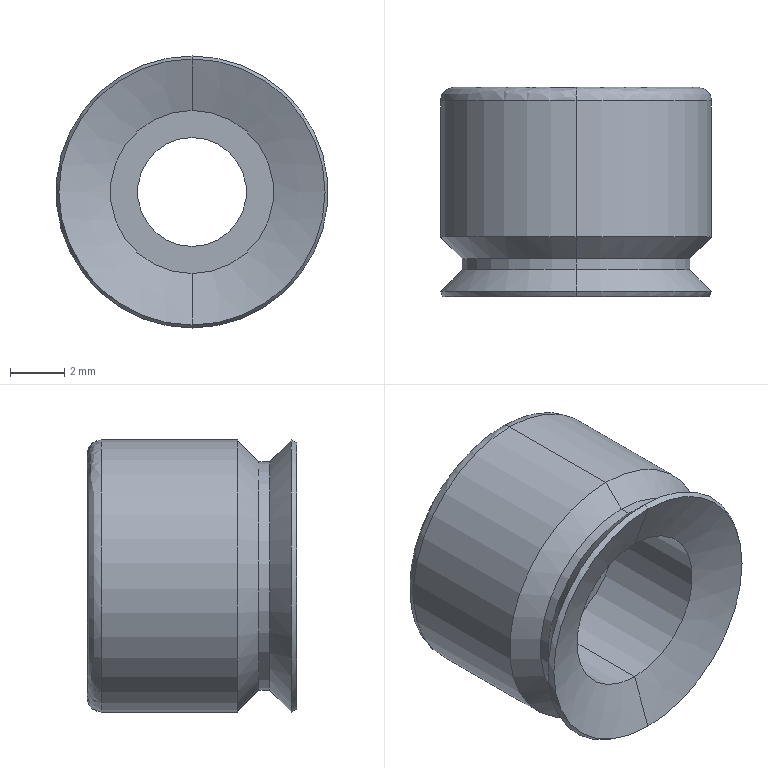Part | STEP file | _J-WES26-d10-003 | 1 solid | 20 faces | box 10 x 7.688 x 10 mm | volume 388.501 mm3 | cylinder 8 | cone 8 | spline 2 | plane 2 | commonest cylinder face diameters 4 x2 6 x2 8.4 x2 10 x2
STEP:
#1=CARTESIAN_POINT('',(0.,8.,4.5));
#2=VERTEX_POINT('',#1);
#3=CARTESIAN_POINT('',(0.,8.,-4.5));
#4=VERTEX_POINT('',#3);
#5=CARTESIAN_POINT('',(0.,8.,4.5));
#6=CARTESIAN_POINT('',(-9.,8.,4.5));
#7=CARTESIAN_POINT('',(-9.,8.,-4.5));
#8=CARTESIAN_POINT('',(0.,8.,-4.5));
#9=(BOUNDED_CURVE()B_SPLINE_CURVE(3,(#5,#6,#7,#8),.UNSPECIFIED.,.F.,.F.)B_SPLINE_CURVE_WITH_KNOTS((4,4),(0.,0.5),.UNSPECIFIED.)CURVE()GEOMETRIC_REPRESENTATION_ITEM()RATIONAL_B_SPLINE_CURVE((1.,0.3333,0.3333,1.))REPRESENTATION_ITEM(''));
#10=EDGE_CURVE('',#2,#4,#9,.T.);
#11=ORIENTED_EDGE('',*,*,#10,.T.);
#12=CARTESIAN_POINT('',(0.,7.5,-5.));
#13=VERTEX_POINT('',#12);
#14=CARTESIAN_POINT('',(0.,7.5,-4.5));
#15=DIRECTION('',(-1.,0.,0.));
#16=DIRECTION('',(0.,0.,-1.));
#17=AXIS2_PLACEMENT_3D('',#14,#15,#16);
#18=CIRCLE('',#17,0.5);
#19=EDGE_CURVE('',#4,#13,#18,.T.);
#20=ORIENTED_EDGE('',*,*,#19,.T.);
#21=CARTESIAN_POINT('',(0.,7.5,5.));
#22=VERTEX_POINT('',#21);
#23=CARTESIAN_POINT('',(0.,7.5,0.));
#24=DIRECTION('',(0.,-1.,0.));
#25=DIRECTION('',(0.,0.,-1.));
#26=AXIS2_PLACEMENT_3D('',#23,#24,#25);
#27=CIRCLE('',#26,5.);
#28=EDGE_CURVE('',#22,#13,#27,.T.);
#29=ORIENTED_EDGE('',*,*,#28,.F.);
#30=CARTESIAN_POINT('',(0.,7.5,4.5));
#31=DIRECTION('',(1.,0.,0.));
#32=DIRECTION('',(0.,0.,1.));
#33=AXIS2_PLACEMENT_3D('',#30,#31,#32);
#34=CIRCLE('',#33,0.5);
#35=EDGE_CURVE('',#2,#22,#34,.T.);
#36=ORIENTED_EDGE('',*,*,#35,.F.);
#37=EDGE_LOOP('',(#11,#20,#29,#36));
#38=FACE_OUTER_BOUND('',#37,.T.);
#39=CARTESIAN_POINT('',(0.,8.,-4.5));
#40=CARTESIAN_POINT('',(-9.,8.,-4.5));
#41=CARTESIAN_POINT('',(-9.,8.,4.5));
#42=CARTESIAN_POINT('',(0.,8.,4.5));
#43=CARTESIAN_POINT('',(0.,8.,-4.793));
#44=CARTESIAN_POINT('',(-9.586,8.,-4.793));
#45=CARTESIAN_POINT('',(-9.586,8.,4.793));
#46=CARTESIAN_POINT('',(0.,8.,4.793));
#47=CARTESIAN_POINT('',(0.,7.793,-5.));
#48=CARTESIAN_POINT('',(-10.,7.793,-5.));
#49=CARTESIAN_POINT('',(-10.,7.793,5.));
#50=CARTESIAN_POINT('',(0.,7.793,5.));
#51=CARTESIAN_POINT('',(0.,7.5,-5.));
#52=CARTESIAN_POINT('',(-10.,7.5,-5.));
#53=CARTESIAN_POINT('',(-10.,7.5,5.));
#54=CARTESIAN_POINT('',(0.,7.5,5.));
#55=(BOUNDED_SURFACE()B_SPLINE_SURFACE(3,3,((#39,#40,#41,#42),(#43,#44,#45,#46),(#47,#48,#49,#50),(#51,#52,#53,#54)),.UNSPECIFIED.,.F.,.F.,.F.)B_SPLINE_SURFACE_WITH_KNOTS((4,4),(4,4),(0.,1.),(0.,1.),.UNSPECIFIED.)GEOMETRIC_REPRESENTATION_ITEM()RATIONAL_B_SPLINE_SURFACE(((1.,0.3333,0.3333,1.),(0.8047,0.2682,0.2682,0.8047),(0.8047,0.2682,0.2682,0.8047),(1.,0.3333,0.3333,1.)))REPRESENTATION_ITEM('')SURFACE());
#56=ADVANCED_FACE('',(#38),#55,.T.);
#57=CARTESIAN_POINT('',(0.,7.5,0.));
#58=DIRECTION('',(0.,-1.,0.));
#59=DIRECTION('',(0.,0.,-1.));
#60=AXIS2_PLACEMENT_3D('',#57,#58,#59);
#61=CIRCLE('',#60,5.);
#62=EDGE_CURVE('',#13,#22,#61,.T.);
#63=ORIENTED_EDGE('',*,*,#62,.T.);
#64=CARTESIAN_POINT('',(0.,2.5,5.));
#65=VERTEX_POINT('',#64);
#66=CARTESIAN_POINT('',(0.,50.,5.));
#67=DIRECTION('',(0.,-1.,0.));
#68=VECTOR('',#67,1000.);
#69=LINE('',#66,#68);
#70=EDGE_CURVE('',#22,#65,#69,.T.);
#71=ORIENTED_EDGE('',*,*,#70,.T.);
#72=CARTESIAN_POINT('',(0.,2.5,-5.));
#73=VERTEX_POINT('',#72);
#74=CARTESIAN_POINT('',(0.,2.5,0.));
#75=DIRECTION('',(0.,1.,0.));
#76=DIRECTION('',(0.,0.,-1.));
#77=AXIS2_PLACEMENT_3D('',#74,#75,#76);
#78=CIRCLE('',#77,5.);
#79=EDGE_CURVE('',#65,#73,#78,.T.);
#80=ORIENTED_EDGE('',*,*,#79,.T.);
#81=CARTESIAN_POINT('',(0.,50.,-5.));
#82=DIRECTION('',(0.,-1.,0.));
#83=VECTOR('',#82,1000.);
#84=LINE('',#81,#83);
#85=EDGE_CURVE('',#13,#73,#84,.T.);
#86=ORIENTED_EDGE('',*,*,#85,.F.);
#87=EDGE_LOOP('',(#63,#71,#80,#86));
#88=FACE_OUTER_BOUND('',#87,.T.);
#89=CARTESIAN_POINT('',(0.,50.,0.));
#90=DIRECTION('',(0.,-1.,0.));
#91=DIRECTION('',(0.,0.,-1.));
#92=AXIS2_PLACEMENT_3D('',#89,#90,#91);
#93=CYLINDRICAL_SURFACE('',#92,5.);
#94=ADVANCED_FACE('',(#88),#93,.T.);
#95=CARTESIAN_POINT('',(0.,1.7,4.2));
#96=VERTEX_POINT('',#95);
#97=CARTESIAN_POINT('',(0.,1.7,-4.2));
#98=VERTEX_POINT('',#97);
#99=CARTESIAN_POINT('',(0.,1.7,0.));
#100=DIRECTION('',(0.,1.,0.));
#101=DIRECTION('',(0.,0.,1.));
#102=AXIS2_PLACEMENT_3D('',#99,#100,#101);
#103=CIRCLE('',#102,4.2);
#104=EDGE_CURVE('',#96,#98,#103,.T.);
#105=ORIENTED_EDGE('',*,*,#104,.T.);
#106=CARTESIAN_POINT('',(0.,2.5,-5.));
#107=DIRECTION('',(0.,0.7071,-0.7071));
#108=VECTOR('',#107,1000.);
#109=LINE('',#106,#108);
#110=EDGE_CURVE('',#98,#73,#109,.T.);
#111=ORIENTED_EDGE('',*,*,#110,.T.);
#112=ORIENTED_EDGE('',*,*,#79,.F.);
#113=CARTESIAN_POINT('',(0.,2.5,5.));
#114=DIRECTION('',(0.,0.7071,0.7071));
#115=VECTOR('',#114,1000.);
#116=LINE('',#113,#115);
#117=EDGE_CURVE('',#96,#65,#116,.T.);
#118=ORIENTED_EDGE('',*,*,#117,.F.);
#119=EDGE_LOOP('',(#105,#111,#112,#118));
#120=FACE_OUTER_BOUND('',#119,.T.);
#121=CARTESIAN_POINT('',(0.,2.5,0.));
#122=DIRECTION('',(0.,1.,0.));
#123=DIRECTION('',(0.,0.,1.));
#124=AXIS2_PLACEMENT_3D('',#121,#122,#123);
#125=CONICAL_SURFACE('',#124,5.,0.7854);
#126=ADVANCED_FACE('',(#120),#125,.T.);
#127=ORIENTED_EDGE('',*,*,#104,.F.);
#128=CARTESIAN_POINT('',(0.,1.3,4.2));
#129=VERTEX_POINT('',#128);
#130=CARTESIAN_POINT('',(0.,50.,4.2));
#131=DIRECTION('',(0.,-1.,0.));
#132=VECTOR('',#131,1000.);
#133=LINE('',#130,#132);
#134=EDGE_CURVE('',#96,#129,#133,.T.);
#135=ORIENTED_EDGE('',*,*,#134,.T.);
#136=CARTESIAN_POINT('',(0.,1.3,-4.2));
#137=VERTEX_POINT('',#136);
#138=CARTESIAN_POINT('',(0.,1.3,0.));
#139=DIRECTION('',(0.,1.,0.));
#140=DIRECTION('',(0.,0.,-1.));
#141=AXIS2_PLACEMENT_3D('',#138,#139,#140);
#142=CIRCLE('',#141,4.2);
#143=EDGE_CURVE('',#129,#137,#142,.T.);
#144=ORIENTED_EDGE('',*,*,#143,.T.);
#145=CARTESIAN_POINT('',(0.,50.,-4.2));
#146=DIRECTION('',(0.,-1.,0.));
#147=VECTOR('',#146,1000.);
#148=LINE('',#145,#147);
#149=EDGE_CURVE('',#98,#137,#148,.T.);
#150=ORIENTED_EDGE('',*,*,#149,.F.);
#151=EDGE_LOOP('',(#127,#135,#144,#150));
#152=FACE_OUTER_BOUND('',#151,.T.);
#153=CARTESIAN_POINT('',(0.,50.,0.));
#154=DIRECTION('',(0.,-1.,0.));
#155=DIRECTION('',(0.,0.,-1.));
#156=AXIS2_PLACEMENT_3D('',#153,#154,#155);
#157=CYLINDRICAL_SURFACE('',#156,4.2);
#158=ADVANCED_FACE('',(#152),#157,.T.);
#159=ORIENTED_EDGE('',*,*,#143,.F.);
#160=CARTESIAN_POINT('',(0.,0.5,5.));
#161=VERTEX_POINT('',#160);
#162=CARTESIAN_POINT('',(0.,0.5,5.));
#163=DIRECTION('',(0.,-0.7071,0.7071));
#164=VECTOR('',#163,1000.);
#165=LINE('',#162,#164);
#166=EDGE_CURVE('',#129,#161,#165,.T.);
#167=ORIENTED_EDGE('',*,*,#166,.T.);
#168=CARTESIAN_POINT('',(0.,0.5,-5.));
#169=VERTEX_POINT('',#168);
#170=CARTESIAN_POINT('',(0.,0.5,0.));
#171=DIRECTION('',(0.,1.,0.));
#172=DIRECTION('',(0.,0.,-1.));
#173=AXIS2_PLACEMENT_3D('',#170,#171,#172);
#174=CIRCLE('',#173,5.);
#175=EDGE_CURVE('',#161,#169,#174,.T.);
#176=ORIENTED_EDGE('',*,*,#175,.T.);
#177=CARTESIAN_POINT('',(0.,0.5,-5.));
#178=DIRECTION('',(0.,-0.7071,-0.7071));
#179=VECTOR('',#178,1000.);
#180=LINE('',#177,#179);
#181=EDGE_CURVE('',#137,#169,#180,.T.);
#182=ORIENTED_EDGE('',*,*,#181,.F.);
#183=EDGE_LOOP('',(#159,#167,#176,#182));
#184=FACE_OUTER_BOUND('',#183,.T.);
#185=CARTESIAN_POINT('',(0.,0.5,0.));
#186=DIRECTION('',(0.,-1.,0.));
#187=DIRECTION('',(0.,0.,-1.));
#188=AXIS2_PLACEMENT_3D('',#185,#186,#187);
#189=CONICAL_SURFACE('',#188,5.,0.7854);
#190=ADVANCED_FACE('',(#184),#189,.T.);
#191=CARTESIAN_POINT('',(0.,8.,-2.));
#192=VERTEX_POINT('',#191);
#193=CARTESIAN_POINT('',(0.,8.,2.));
#194=VERTEX_POINT('',#193);
#195=CARTESIAN_POINT('',(0.,8.,0.));
#196=DIRECTION('',(0.,1.,0.));
#197=DIRECTION('',(0.,0.,-1.));
#198=AXIS2_PLACEMENT_3D('',#195,#196,#197);
#199=CIRCLE('',#198,2.);
#200=EDGE_CURVE('',#192,#194,#199,.T.);
#201=ORIENTED_EDGE('',*,*,#200,.T.);
#202=CARTESIAN_POINT('',(0.,5.,2.));
#203=VERTEX_POINT('',#202);
#204=CARTESIAN_POINT('',(0.,50.,2.));
#205=DIRECTION('',(0.,-1.,0.));
#206=VECTOR('',#205,1000.);
#207=LINE('',#204,#206);
#208=EDGE_CURVE('',#194,#203,#207,.T.);
#209=ORIENTED_EDGE('',*,*,#208,.T.);
#210=CARTESIAN_POINT('',(0.,5.,-2.));
#211=VERTEX_POINT('',#210);
#212=CARTESIAN_POINT('',(0.,5.,0.));
#213=DIRECTION('',(0.,1.,0.));
#214=DIRECTION('',(0.,0.,-1.));
#215=AXIS2_PLACEMENT_3D('',#212,#213,#214);
#216=CIRCLE('',#215,2.);
#217=EDGE_CURVE('',#211,#203,#216,.T.);
#218=ORIENTED_EDGE('',*,*,#217,.F.);
#219=CARTESIAN_POINT('',(0.,50.,-2.));
#220=DIRECTION('',(0.,-1.,0.));
#221=VECTOR('',#220,1000.);
#222=LINE('',#219,#221);
#223=EDGE_CURVE('',#192,#211,#222,.T.);
#224=ORIENTED_EDGE('',*,*,#223,.F.);
#225=EDGE_LOOP('',(#201,#209,#218,#224));
#226=FACE_OUTER_BOUND('',#225,.T.);
#227=CARTESIAN_POINT('',(0.,50.,0.));
#228=DIRECTION('',(0.,-1.,0.));
#229=DIRECTION('',(0.,0.,-1.));
#230=AXIS2_PLACEMENT_3D('',#227,#228,#229);
#231=CYLINDRICAL_SURFACE('',#230,2.);
#232=ADVANCED_FACE('',(#226),#231,.F.);
#233=CARTESIAN_POINT('',(0.,0.3116,4.891));
#234=VERTEX_POINT('',#233);
#235=CARTESIAN_POINT('',(0.,0.3116,-4.891));
#236=VERTEX_POINT('',#235);
#237=CARTESIAN_POINT('',(0.,0.3116,0.));
#238=DIRECTION('',(0.,1.,0.));
#239=DIRECTION('',(0.,0.,1.));
#240=AXIS2_PLACEMENT_3D('',#237,#238,#239);
#241=CIRCLE('',#240,4.891);
#242=EDGE_CURVE('',#234,#236,#241,.T.);
#243=ORIENTED_EDGE('',*,*,#242,.T.);
#244=CARTESIAN_POINT('',(0.,0.5,-5.));
#245=DIRECTION('',(0.,0.866,-0.5));
#246=VECTOR('',#245,1000.);
#247=LINE('',#244,#246);
#248=EDGE_CURVE('',#236,#169,#247,.T.);
#249=ORIENTED_EDGE('',*,*,#248,.T.);
#250=ORIENTED_EDGE('',*,*,#175,.F.);
#251=CARTESIAN_POINT('',(0.,0.5,5.));
#252=DIRECTION('',(0.,0.866,0.5));
#253=VECTOR('',#252,1000.);
#254=LINE('',#251,#253);
#255=EDGE_CURVE('',#234,#161,#254,.T.);
#256=ORIENTED_EDGE('',*,*,#255,.F.);
#257=EDGE_LOOP('',(#243,#249,#250,#256));
#258=FACE_OUTER_BOUND('',#257,.T.);
#259=CARTESIAN_POINT('',(0.,0.5,0.));
#260=DIRECTION('',(0.,1.,0.));
#261=DIRECTION('',(0.,0.,1.));
#262=AXIS2_PLACEMENT_3D('',#259,#260,#261);
#263=CONICAL_SURFACE('',#262,5.,0.5236);
#264=ADVANCED_FACE('',(#258),#263,.T.);
#265=CARTESIAN_POINT('',(0.,1.,3.));
#266=VERTEX_POINT('',#265);
#267=CARTESIAN_POINT('',(0.,1.,-3.));
#268=VERTEX_POINT('',#267);
#269=CARTESIAN_POINT('',(0.,1.,0.));
#270=DIRECTION('',(0.,-1.,0.));
#271=DIRECTION('',(0.,0.,-1.));
#272=AXIS2_PLACEMENT_3D('',#269,#270,#271);
#273=CIRCLE('',#272,3.);
#274=EDGE_CURVE('',#266,#268,#273,.T.);
#275=ORIENTED_EDGE('',*,*,#274,.F.);
#276=CARTESIAN_POINT('',(0.,0.3116,4.891));
#277=DIRECTION('',(0.,-0.342,0.9397));
#278=VECTOR('',#277,1000.);
#279=LINE('',#276,#278);
#280=EDGE_CURVE('',#266,#234,#279,.T.);
#281=ORIENTED_EDGE('',*,*,#280,.T.);
#282=CARTESIAN_POINT('',(0.,0.3116,0.));
#283=DIRECTION('',(0.,1.,0.));
#284=DIRECTION('',(0.,0.,1.));
#285=AXIS2_PLACEMENT_3D('',#282,#283,#284);
#286=CIRCLE('',#285,4.891);
#287=EDGE_CURVE('',#236,#234,#286,.T.);
#288=ORIENTED_EDGE('',*,*,#287,.F.);
#289=CARTESIAN_POINT('',(0.,0.3116,-4.891));
#290=DIRECTION('',(0.,-0.342,-0.9397));
#291=VECTOR('',#290,1000.);
#292=LINE('',#289,#291);
#293=EDGE_CURVE('',#268,#236,#292,.T.);
#294=ORIENTED_EDGE('',*,*,#293,.F.);
#295=EDGE_LOOP('',(#275,#281,#288,#294));
#296=FACE_OUTER_BOUND('',#295,.T.);
#297=CARTESIAN_POINT('',(0.,0.3116,0.));
#298=DIRECTION('',(0.,-1.,0.));
#299=DIRECTION('',(0.,0.,-1.));
#300=AXIS2_PLACEMENT_3D('',#297,#298,#299);
#301=CONICAL_SURFACE('',#300,4.891,1.222);
#302=ADVANCED_FACE('',(#296),#301,.F.);
#303=CARTESIAN_POINT('',(0.,5.,3.));
#304=VERTEX_POINT('',#303);
#305=CARTESIAN_POINT('',(0.,5.,-3.));
#306=VERTEX_POINT('',#305);
#307=CARTESIAN_POINT('',(0.,5.,0.));
#308=DIRECTION('',(0.,-1.,0.));
#309=DIRECTION('',(0.,0.,-1.));
#310=AXIS2_PLACEMENT_3D('',#307,#308,#309);
#311=CIRCLE('',#310,3.);
#312=EDGE_CURVE('',#304,#306,#311,.T.);
#313=ORIENTED_EDGE('',*,*,#312,.F.);
#314=CARTESIAN_POINT('',(0.,50.,3.));
#315=DIRECTION('',(0.,-1.,0.));
#316=VECTOR('',#315,1000.);
#317=LINE('',#314,#316);
#318=EDGE_CURVE('',#304,#266,#317,.T.);
#319=ORIENTED_EDGE('',*,*,#318,.T.);
#320=ORIENTED_EDGE('',*,*,#274,.T.);
#321=CARTESIAN_POINT('',(0.,50.,-3.));
#322=DIRECTION('',(0.,-1.,0.));
#323=VECTOR('',#322,1000.);
#324=LINE('',#321,#323);
#325=EDGE_CURVE('',#306,#268,#324,.T.);
#326=ORIENTED_EDGE('',*,*,#325,.F.);
#327=EDGE_LOOP('',(#313,#319,#320,#326));
#328=FACE_OUTER_BOUND('',#327,.T.);
#329=CARTESIAN_POINT('',(0.,50.,0.));
#330=DIRECTION('',(0.,-1.,0.));
#331=DIRECTION('',(0.,0.,-1.));
#332=AXIS2_PLACEMENT_3D('',#329,#330,#331);
#333=CYLINDRICAL_SURFACE('',#332,3.);
#334=ADVANCED_FACE('',(#328),#333,.F.);
#335=ORIENTED_EDGE('',*,*,#70,.F.);
#336=ORIENTED_EDGE('',*,*,#28,.T.);
#337=ORIENTED_EDGE('',*,*,#85,.T.);
#338=CARTESIAN_POINT('',(0.,2.5,0.));
#339=DIRECTION('',(0.,1.,0.));
#340=DIRECTION('',(0.,0.,-1.));
#341=AXIS2_PLACEMENT_3D('',#338,#339,#340);
#342=CIRCLE('',#341,5.);
#343=EDGE_CURVE('',#73,#65,#342,.T.);
#344=ORIENTED_EDGE('',*,*,#343,.T.);
#345=EDGE_LOOP('',(#335,#336,#337,#344));
#346=FACE_OUTER_BOUND('',#345,.T.);
#347=CARTESIAN_POINT('',(0.,50.,0.));
#348=DIRECTION('',(0.,-1.,0.));
#349=DIRECTION('',(0.,0.,-1.));
#350=AXIS2_PLACEMENT_3D('',#347,#348,#349);
#351=CYLINDRICAL_SURFACE('',#350,5.);
#352=ADVANCED_FACE('',(#346),#351,.T.);
#353=ORIENTED_EDGE('',*,*,#110,.F.);
#354=CARTESIAN_POINT('',(0.,1.7,0.));
#355=DIRECTION('',(0.,1.,0.));
#356=DIRECTION('',(0.,0.,1.));
#357=AXIS2_PLACEMENT_3D('',#354,#355,#356);
#358=CIRCLE('',#357,4.2);
#359=EDGE_CURVE('',#98,#96,#358,.T.);
#360=ORIENTED_EDGE('',*,*,#359,.T.);
#361=ORIENTED_EDGE('',*,*,#117,.T.);
#362=ORIENTED_EDGE('',*,*,#343,.F.);
#363=EDGE_LOOP('',(#353,#360,#361,#362));
#364=FACE_OUTER_BOUND('',#363,.T.);
#365=CARTESIAN_POINT('',(0.,2.5,0.));
#366=DIRECTION('',(0.,1.,0.));
#367=DIRECTION('',(0.,0.,1.));
#368=AXIS2_PLACEMENT_3D('',#365,#366,#367);
#369=CONICAL_SURFACE('',#368,5.,0.7854);
#370=ADVANCED_FACE('',(#364),#369,.T.);
#371=ORIENTED_EDGE('',*,*,#19,.F.);
#372=CARTESIAN_POINT('',(0.,8.,-4.5));
#373=CARTESIAN_POINT('',(9.,8.,-4.5));
#374=CARTESIAN_POINT('',(9.,8.,4.5));
#375=CARTESIAN_POINT('',(0.,8.,4.5));
#376=(BOUNDED_CURVE()B_SPLINE_CURVE(3,(#372,#373,#374,#375),.UNSPECIFIED.,.F.,.F.)B_SPLINE_CURVE_WITH_KNOTS((4,4),(0.5,1.),.UNSPECIFIED.)CURVE()GEOMETRIC_REPRESENTATION_ITEM()RATIONAL_B_SPLINE_CURVE((1.,0.3333,0.3333,1.))REPRESENTATION_ITEM(''));
#377=EDGE_CURVE('',#4,#2,#376,.T.);
#378=ORIENTED_EDGE('',*,*,#377,.T.);
#379=ORIENTED_EDGE('',*,*,#35,.T.);
#380=ORIENTED_EDGE('',*,*,#62,.F.);
#381=EDGE_LOOP('',(#371,#378,#379,#380));
#382=FACE_OUTER_BOUND('',#381,.T.);
#383=CARTESIAN_POINT('',(0.,8.,4.5));
#384=CARTESIAN_POINT('',(9.,8.,4.5));
#385=CARTESIAN_POINT('',(9.,8.,-4.5));
#386=CARTESIAN_POINT('',(0.,8.,-4.5));
#387=CARTESIAN_POINT('',(0.,8.,4.793));
#388=CARTESIAN_POINT('',(9.586,8.,4.793));
#389=CARTESIAN_POINT('',(9.586,8.,-4.793));
#390=CARTESIAN_POINT('',(0.,8.,-4.793));
#391=CARTESIAN_POINT('',(0.,7.793,5.));
#392=CARTESIAN_POINT('',(10.,7.793,5.));
#393=CARTESIAN_POINT('',(10.,7.793,-5.));
#394=CARTESIAN_POINT('',(0.,7.793,-5.));
#395=CARTESIAN_POINT('',(0.,7.5,5.));
#396=CARTESIAN_POINT('',(10.,7.5,5.));
#397=CARTESIAN_POINT('',(10.,7.5,-5.));
#398=CARTESIAN_POINT('',(0.,7.5,-5.));
#399=(BOUNDED_SURFACE()B_SPLINE_SURFACE(3,3,((#383,#384,#385,#386),(#387,#388,#389,#390),(#391,#392,#393,#394),(#395,#396,#397,#398)),.UNSPECIFIED.,.F.,.F.,.T.)B_SPLINE_SURFACE_WITH_KNOTS((4,4),(4,4),(0.,1.),(0.,1.),.UNSPECIFIED.)GEOMETRIC_REPRESENTATION_ITEM()RATIONAL_B_SPLINE_SURFACE(((1.,0.3333,0.3333,1.),(0.8047,0.2682,0.2682,0.8047),(0.8047,0.2682,0.2682,0.8047),(1.,0.3333,0.3333,1.)))REPRESENTATION_ITEM('')SURFACE());
#400=ADVANCED_FACE('',(#382),#399,.T.);
#401=ORIENTED_EDGE('',*,*,#134,.F.);
#402=ORIENTED_EDGE('',*,*,#359,.F.);
#403=ORIENTED_EDGE('',*,*,#149,.T.);
#404=CARTESIAN_POINT('',(0.,1.3,0.));
#405=DIRECTION('',(0.,1.,0.));
#406=DIRECTION('',(0.,0.,-1.));
#407=AXIS2_PLACEMENT_3D('',#404,#405,#406);
#408=CIRCLE('',#407,4.2);
#409=EDGE_CURVE('',#137,#129,#408,.T.);
#410=ORIENTED_EDGE('',*,*,#409,.T.);
#411=EDGE_LOOP('',(#401,#402,#403,#410));
#412=FACE_OUTER_BOUND('',#411,.T.);
#413=CARTESIAN_POINT('',(0.,50.,0.));
#414=DIRECTION('',(0.,-1.,0.));
#415=DIRECTION('',(0.,0.,-1.));
#416=AXIS2_PLACEMENT_3D('',#413,#414,#415);
#417=CYLINDRICAL_SURFACE('',#416,4.2);
#418=ADVANCED_FACE('',(#412),#417,.T.);
#419=ORIENTED_EDGE('',*,*,#10,.F.);
#420=ORIENTED_EDGE('',*,*,#377,.F.);
#421=EDGE_LOOP('',(#419,#420));
#422=FACE_OUTER_BOUND('',#421,.T.);
#423=ORIENTED_EDGE('',*,*,#200,.F.);
#424=CARTESIAN_POINT('',(0.,8.,0.));
#425=DIRECTION('',(0.,1.,0.));
#426=DIRECTION('',(0.,0.,-1.));
#427=AXIS2_PLACEMENT_3D('',#424,#425,#426);
#428=CIRCLE('',#427,2.);
#429=EDGE_CURVE('',#194,#192,#428,.T.);
#430=ORIENTED_EDGE('',*,*,#429,.F.);
#431=EDGE_LOOP('',(#423,#430));
#432=FACE_BOUND('',#431,.T.);
#433=CARTESIAN_POINT('',(0.,8.,4.5));
#434=DIRECTION('',(0.,-1.,0.));
#435=DIRECTION('',(0.,0.,-1.));
#436=AXIS2_PLACEMENT_3D('',#433,#434,#435);
#437=PLANE('',#436);
#438=ADVANCED_FACE('',(#422,#432),#437,.F.);
#439=ORIENTED_EDGE('',*,*,#166,.F.);
#440=ORIENTED_EDGE('',*,*,#409,.F.);
#441=ORIENTED_EDGE('',*,*,#181,.T.);
#442=CARTESIAN_POINT('',(0.,0.5,0.));
#443=DIRECTION('',(0.,1.,0.));
#444=DIRECTION('',(0.,0.,-1.));
#445=AXIS2_PLACEMENT_3D('',#442,#443,#444);
#446=CIRCLE('',#445,5.);
#447=EDGE_CURVE('',#169,#161,#446,.T.);
#448=ORIENTED_EDGE('',*,*,#447,.T.);
#449=EDGE_LOOP('',(#439,#440,#441,#448));
#450=FACE_OUTER_BOUND('',#449,.T.);
#451=CARTESIAN_POINT('',(0.,0.5,0.));
#452=DIRECTION('',(0.,-1.,0.));
#453=DIRECTION('',(0.,0.,-1.));
#454=AXIS2_PLACEMENT_3D('',#451,#452,#453);
#455=CONICAL_SURFACE('',#454,5.,0.7854);
#456=ADVANCED_FACE('',(#450),#455,.T.);
#457=ORIENTED_EDGE('',*,*,#208,.F.);
#458=ORIENTED_EDGE('',*,*,#429,.T.);
#459=ORIENTED_EDGE('',*,*,#223,.T.);
#460=CARTESIAN_POINT('',(0.,5.,0.));
#461=DIRECTION('',(0.,1.,0.));
#462=DIRECTION('',(0.,0.,-1.));
#463=AXIS2_PLACEMENT_3D('',#460,#461,#462);
#464=CIRCLE('',#463,2.);
#465=EDGE_CURVE('',#203,#211,#464,.T.);
#466=ORIENTED_EDGE('',*,*,#465,.F.);
#467=EDGE_LOOP('',(#457,#458,#459,#466));
#468=FACE_OUTER_BOUND('',#467,.T.);
#469=CARTESIAN_POINT('',(0.,50.,0.));
#470=DIRECTION('',(0.,-1.,0.));
#471=DIRECTION('',(0.,0.,-1.));
#472=AXIS2_PLACEMENT_3D('',#469,#470,#471);
#473=CYLINDRICAL_SURFACE('',#472,2.);
#474=ADVANCED_FACE('',(#468),#473,.F.);
#475=ORIENTED_EDGE('',*,*,#248,.F.);
#476=ORIENTED_EDGE('',*,*,#287,.T.);
#477=ORIENTED_EDGE('',*,*,#255,.T.);
#478=ORIENTED_EDGE('',*,*,#447,.F.);
#479=EDGE_LOOP('',(#475,#476,#477,#478));
#480=FACE_OUTER_BOUND('',#479,.T.);
#481=CARTESIAN_POINT('',(0.,0.5,0.));
#482=DIRECTION('',(0.,1.,0.));
#483=DIRECTION('',(0.,0.,1.));
#484=AXIS2_PLACEMENT_3D('',#481,#482,#483);
#485=CONICAL_SURFACE('',#484,5.,0.5236);
#486=ADVANCED_FACE('',(#480),#485,.T.);
#487=CARTESIAN_POINT('',(0.,5.,0.));
#488=DIRECTION('',(0.,-1.,0.));
#489=DIRECTION('',(0.,0.,-1.));
#490=AXIS2_PLACEMENT_3D('',#487,#488,#489);
#491=CIRCLE('',#490,3.);
#492=EDGE_CURVE('',#306,#304,#491,.T.);
#493=ORIENTED_EDGE('',*,*,#492,.T.);
#494=ORIENTED_EDGE('',*,*,#312,.T.);
#495=EDGE_LOOP('',(#493,#494));
#496=FACE_OUTER_BOUND('',#495,.T.);
#497=ORIENTED_EDGE('',*,*,#217,.T.);
#498=ORIENTED_EDGE('',*,*,#465,.T.);
#499=EDGE_LOOP('',(#497,#498));
#500=FACE_BOUND('',#499,.T.);
#501=CARTESIAN_POINT('',(0.,5.,3.));
#502=DIRECTION('',(0.,-1.,0.));
#503=DIRECTION('',(0.,0.,-1.));
#504=AXIS2_PLACEMENT_3D('',#501,#502,#503);
#505=PLANE('',#504);
#506=ADVANCED_FACE('',(#496,#500),#505,.T.);
#507=ORIENTED_EDGE('',*,*,#280,.F.);
#508=CARTESIAN_POINT('',(0.,1.,0.));
#509=DIRECTION('',(0.,-1.,0.));
#510=DIRECTION('',(0.,0.,-1.));
#511=AXIS2_PLACEMENT_3D('',#508,#509,#510);
#512=CIRCLE('',#511,3.);
#513=EDGE_CURVE('',#268,#266,#512,.T.);
#514=ORIENTED_EDGE('',*,*,#513,.F.);
#515=ORIENTED_EDGE('',*,*,#293,.T.);
#516=ORIENTED_EDGE('',*,*,#242,.F.);
#517=EDGE_LOOP('',(#507,#514,#515,#516));
#518=FACE_OUTER_BOUND('',#517,.T.);
#519=CARTESIAN_POINT('',(0.,0.3116,0.));
#520=DIRECTION('',(0.,-1.,0.));
#521=DIRECTION('',(0.,0.,-1.));
#522=AXIS2_PLACEMENT_3D('',#519,#520,#521);
#523=CONICAL_SURFACE('',#522,4.891,1.222);
#524=ADVANCED_FACE('',(#518),#523,.F.);
#525=ORIENTED_EDGE('',*,*,#318,.F.);
#526=ORIENTED_EDGE('',*,*,#492,.F.);
#527=ORIENTED_EDGE('',*,*,#325,.T.);
#528=ORIENTED_EDGE('',*,*,#513,.T.);
#529=EDGE_LOOP('',(#525,#526,#527,#528));
#530=FACE_OUTER_BOUND('',#529,.T.);
#531=CARTESIAN_POINT('',(0.,50.,0.));
#532=DIRECTION('',(0.,-1.,0.));
#533=DIRECTION('',(0.,0.,-1.));
#534=AXIS2_PLACEMENT_3D('',#531,#532,#533);
#535=CYLINDRICAL_SURFACE('',#534,3.);
#536=ADVANCED_FACE('',(#530),#535,.F.);
#537=CLOSED_SHELL('',(#56,#94,#126,#158,#190,#232,#264,#302,#334,#352,#370,#400,#418,#438,#456,#474,#486,#506,#524,#536));
#538=MANIFOLD_SOLID_BREP('',#537);
#539=CARTESIAN_POINT('',(0.,0.,0.));
#540=DIRECTION('',(0.,0.,1.));
#541=DIRECTION('',(1.,0.,0.));
#542=AXIS2_PLACEMENT_3D('',#539,#540,#541);
#543=(LENGTH_UNIT()NAMED_UNIT(*)SI_UNIT(.MILLI.,.METRE.));
#544=UNCERTAINTY_MEASURE_WITH_UNIT(LENGTH_MEASURE(0.00001),#543,'','');
#545=(NAMED_UNIT(*)PLANE_ANGLE_UNIT()SI_UNIT($,.RADIAN.));
#546=(NAMED_UNIT(*)SI_UNIT($,.STERADIAN.)SOLID_ANGLE_UNIT());
#547=(GEOMETRIC_REPRESENTATION_CONTEXT(3)GLOBAL_UNCERTAINTY_ASSIGNED_CONTEXT((#544))GLOBAL_UNIT_ASSIGNED_CONTEXT((#543,#545,#546))REPRESENTATION_CONTEXT('',''));
#548=ADVANCED_BREP_SHAPE_REPRESENTATION('',(#538,#542),#547);